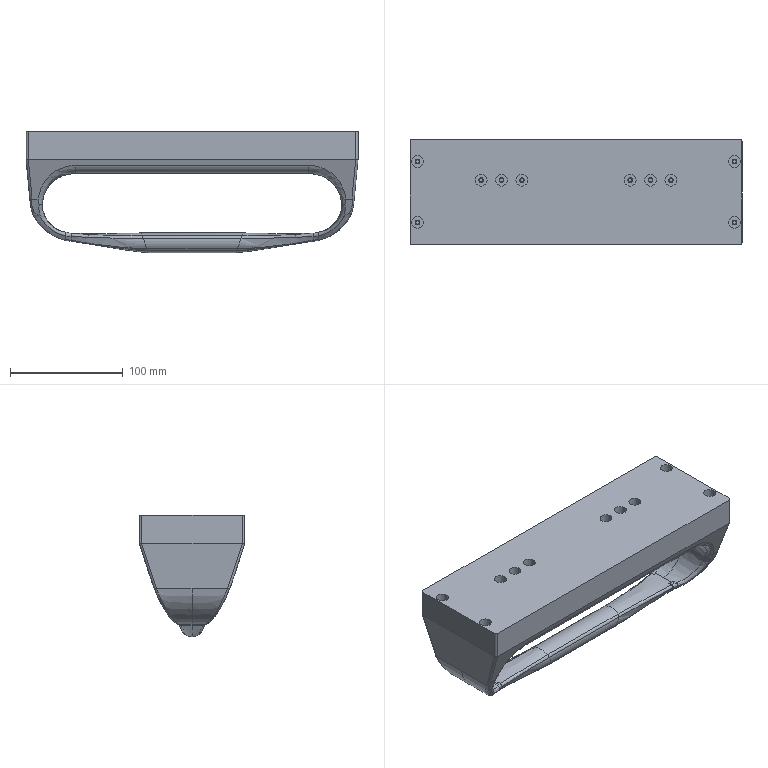NC program | NX | posted with a generic post | part box 294.078 x 93.5 x 107.5 mm
Lines 374 to 1245 of 3753:
(ZLEVEL_PROFILE_COPY_1_COPY_1_COPY_1_1 , TOOL : D6)
N716 T05 M6
N718 G54
N720 G17 G0 G90 X132.194 Y-28.666 B0. C0. S7500 M3
N722 G43 Z28.5 H5
N724 Z-0.05
N726 G94 G1 Z-1.55 F800.
N728 X133.111 Y-28.097
N730 G3 X133.394 Y-27.568 R0.6
N732 G2 X133.414 Y-26.507 R10.372 F3000.
N734 X139.062 Y-20.125 R7.005
N736 G3 X141.389 Y-17.198 R3.024
N738 G1 Y17.198
N740 G3 X138.883 Y20.166 R3.036
N742 G1 X138.816 Y20.183
N744 G2 X133.394 Y27.224 R7.011
N746 G1 Z-1.6
N748 G3 X138.819 Y20.182 R7.011
N750 G1 X138.882 Y20.166
N752 G2 X141.384 Y17.199 R3.035
N754 G1 Y-17.199
N756 G2 X139.062 Y-20.125 R3.024
N758 G3 X133.414 Y-26.507 R7.005
N760 X133.394 Y-27.568 R10.367
N762 G1 Z-1.649
N764 G2 X133.415 Y-26.492 R10.363
N766 X138.873 Y-20.168 R6.993
N768 G1 X139.062 Y-20.125
N770 G3 X141.38 Y-17.2 R3.024
N772 G1 Y17.2
N774 G3 X138.882 Y20.166 R3.034
N776 G1 X138.821 Y20.182
N778 G2 X133.394 Y27.224 R7.011
N780 G1 Z-1.699
N782 G3 X138.824 Y20.181 R7.011
N784 G1 X138.882 Y20.166
N786 G2 X141.375 Y17.201 R3.033
N788 G1 Y-17.201
N790 G2 X139.061 Y-20.125 R3.025
N792 G1 X138.873 Y-20.168
N794 G3 X133.415 Y-26.493 R6.994
N796 X133.394 Y-27.568 R10.358
N798 G1 Z-1.749
N800 G2 X133.415 Y-26.496 R10.384
N802 X138.873 Y-20.168 R6.995
N804 G1 X139.061 Y-20.125
N806 G3 X141.37 Y-17.202 R3.025
N808 G1 Y17.202
N810 G3 X138.881 Y20.166 R3.033
N812 G1 X138.826 Y20.18
N814 G2 X133.394 Y27.224 R7.011
N816 G1 Z-1.799
N818 G3 X138.829 Y20.179 R7.011
N820 G1 X138.881 Y20.166
N822 G2 X141.365 Y17.203 R3.032
N824 G1 Y-17.203
N826 G2 X139.061 Y-20.125 R3.025
N828 G1 X138.873 Y-20.168
N830 G3 X133.415 Y-26.496 R6.995
N832 X133.394 Y-27.568 R10.38
N834 G1 Z-1.848
N836 G2 X133.415 Y-26.496 R10.375
N838 X138.873 Y-20.168 R6.995
N840 G1 X139.061 Y-20.125
N842 G3 X141.361 Y-17.204 R3.025
N844 G1 Y17.204
N846 G3 X138.88 Y20.166 R3.031
N848 G1 X138.831 Y20.179
N850 G2 X133.394 Y27.224 R7.011
N852 G1 Z-1.898
N854 G3 X138.834 Y20.178 R7.011
N856 G1 X138.88 Y20.166
N858 G2 X141.356 Y17.205 R3.03
N860 G1 Y-17.205
N862 G2 X139.06 Y-20.125 R3.025
N864 G1 X138.873 Y-20.168
N866 G3 X133.415 Y-26.496 R6.995
N868 X133.394 Y-27.568 R10.37
N870 G1 Z-1.948
N872 G2 X133.415 Y-26.496 R10.366
N874 X138.873 Y-20.168 R6.995
N876 G1 X139.059 Y-20.125
N878 G3 X141.351 Y-17.206 R3.025
N880 G1 Y17.206
N882 G3 X138.88 Y20.166 R3.03
N884 G1 X138.836 Y20.177
N886 G2 X133.394 Y27.224 R7.011
N888 G1 Z-1.998
N890 G3 X138.839 Y20.176 R7.011
N892 G1 X138.879 Y20.166
N894 G2 X141.346 Y17.207 R3.029
N896 G1 Y-17.207
N898 G2 X139.058 Y-20.125 R3.024
N900 G1 X138.873 Y-20.168
N902 G3 X133.415 Y-26.496 R6.995
N904 X133.394 Y-27.568 R10.361
N906 G1 Z-2.047
N908 G2 X133.415 Y-26.496 R10.356
N910 X138.873 Y-20.168 R6.996
N912 G1 X139.057 Y-20.125
N914 G3 X141.341 Y-17.208 R3.024
N916 G1 Y17.208
N918 G3 X138.879 Y20.166 R3.029
N920 G1 X138.841 Y20.176
N922 G2 X133.394 Y27.224 R7.012
N924 G1 Z-2.097
N926 G3 X138.844 Y20.175 R7.012
N928 G1 X138.878 Y20.166
N930 G2 X141.337 Y17.209 R3.028
N932 G1 Y-17.209
N934 G2 X138.873 Y-20.168 R3.03
N936 G3 X133.415 Y-26.496 R6.996
N938 X133.394 Y-27.568 R10.352
N940 G1 Z-2.147
N942 G2 X133.416 Y-26.488 R10.347
N944 X138.933 Y-20.156 R6.991
N946 G3 X141.332 Y-17.21 R3.03
N948 G1 Y17.21
N950 G3 X138.878 Y20.166 R3.028
N952 G1 X138.846 Y20.174
N954 G2 X133.394 Y27.224 R7.013
N956 G1 Z-2.197
N958 G3 X138.849 Y20.173 R7.013
N960 G1 X138.877 Y20.166
N962 G2 X141.327 Y17.211 R3.027
N964 G1 Y-17.211
N966 G2 X138.93 Y-20.156 R3.029
N968 G3 X133.416 Y-26.488 R6.992
N970 X133.394 Y-27.568 R10.342
N972 G1 Z-2.247
N974 G2 X133.416 Y-26.489 R10.338
N976 X138.927 Y-20.157 R6.992
N978 G3 X141.322 Y-17.212 R3.029
N980 G1 Y17.212
N982 G3 X138.877 Y20.166 R3.026
N984 G1 X138.851 Y20.173
N986 G2 X133.394 Y27.224 R7.014
N988 G1 Z-2.296
N990 G3 X138.877 Y20.166 R7.015
N992 G2 X141.318 Y17.213 R3.026
N994 G1 Y-17.213
N996 G2 X138.924 Y-20.157 R3.029
N998 G3 X133.416 Y-26.489 R6.993
N1000 X133.394 Y-27.568 R10.333
N1002 G1 Z-2.346
N1004 G2 X133.416 Y-26.489 R10.328
N1006 X138.921 Y-20.158 R6.993
N1008 G3 X141.313 Y-17.214 R3.028
N1010 G1 Y17.214
N1012 G3 X138.876 Y20.166 R3.025
N1014 G1 X138.856 Y20.171
N1016 G2 X133.394 Y27.224 R7.015
N1018 G1 Z-2.396
N1020 G3 X138.876 Y20.166 R7.016
N1022 G2 X141.308 Y17.215 R3.025
N1024 G1 Y-17.215
N1026 G2 X138.918 Y-20.158 R3.027
N1028 G3 X133.415 Y-26.49 R6.993
N1030 X133.394 Y-27.568 R10.324
N1032 G1 Z-2.446
N1034 G2 X133.415 Y-26.49 R10.319
N1036 X138.915 Y-20.159 R6.994
N1038 G3 X141.303 Y-17.216 R3.027
N1040 G1 Y17.216
N1042 G3 X138.861 Y20.169 R3.025
N1044 G2 X133.394 Y27.224 R7.016
N1046 G1 Z-2.495
N1048 G3 X138.875 Y20.166 R7.016
N1050 G2 X141.299 Y17.217 R3.024
N1052 G1 Y-17.217
N1054 G2 X138.912 Y-20.159 R3.027
N1056 G3 X133.415 Y-26.491 R6.994
N1058 X133.394 Y-27.568 R10.314
N1060 G1 Z-2.545
N1062 G2 X133.415 Y-26.491 R10.31
N1064 X138.909 Y-20.16 R6.995
N1066 G3 X141.294 Y-17.218 R3.027
N1068 G1 Y17.218
N1070 G3 X138.866 Y20.168 R3.023
N1072 G2 X133.394 Y27.224 R7.017
N1074 G1 Z-2.595
N1076 G3 X138.874 Y20.166 R7.018
N1078 G2 X141.289 Y17.219 R3.022
N1080 G1 Y-17.219
N1082 G2 X138.906 Y-20.16 R3.026
N1084 G3 X133.415 Y-26.492 R6.995
N1086 X133.394 Y-27.568 R10.305
N1088 G1 Z-2.645
N1090 G2 X133.415 Y-26.492 R10.3
N1092 X138.903 Y-20.161 R6.995
N1094 G3 X141.284 Y-17.22 R3.025
N1096 G1 Y17.22
N1098 G3 X138.871 Y20.166 R3.022
N1100 G2 X133.394 Y27.224 R7.018
N1102 G1 Z-2.695
N1104 G3 X138.887 Y20.163 R7.018
N1106 G2 X141.28 Y17.221 R3.021
N1108 G1 Y-17.221
N1110 G2 X138.9 Y-20.161 R3.025
N1112 G3 X133.415 Y-26.493 R6.996
N1114 X133.394 Y-27.568 R10.308
N1116 G1 Z-2.744
N1118 G2 X133.49 Y-25.845 R9.094
N1120 X139.044 Y-20.125 R7.035
N1122 G3 X141.275 Y-17.223 R3.02
N1124 G1 Y17.222
N1126 G3 X138.887 Y20.163 R3.021
N1128 G2 X133.394 Y27.224 R7.017
N1130 G1 Z-2.794
N1132 G3 X138.887 Y20.163 R7.017
N1134 G2 X141.27 Y17.223 R3.02
N1136 G1 Y-17.222
N1138 G2 X141.249 Y-17.572 R2.907
N1140 X139.043 Y-20.125 R3.023
N1142 G3 X133.49 Y-25.845 R7.037
N1144 X133.394 Y-27.568 R9.093
N1146 G1 Z-2.844
N1148 G2 X133.642 Y-25.155 R8.099
N1150 X139.042 Y-20.125 R7.044
N1152 G3 X141.244 Y-17.572 R3.022
N1154 X141.265 Y-17.223 R2.914
N1156 G1 Y17.224
N1158 G3 X138.887 Y20.163 R3.02
N1160 G2 X133.394 Y27.224 R7.017
N1162 G1 Z-2.894
N1164 G3 X138.886 Y20.163 R7.017
N1166 G2 X141.26 Y17.226 R3.019
N1168 G1 Y-17.223
N1170 G2 X141.239 Y-17.575 R2.919
N1172 X139.041 Y-20.125 R3.022
N1174 G3 X133.642 Y-25.155 R7.046
N1176 X133.394 Y-27.568 R8.097
N1178 G1 Z-2.943
N1180 G2 X133.642 Y-25.155 R8.095
N1182 X139.04 Y-20.125 R7.049
N1184 G3 X141.235 Y-17.575 R3.022
N1186 X141.256 Y-17.224 R2.92
N1188 G1 Y17.227
N1190 G3 X138.886 Y20.162 R3.019
N1192 G2 X133.394 Y27.224 R7.019
N1194 G1 Z-2.993
N1196 G3 X138.886 Y20.162 R7.019
N1198 G2 X141.251 Y17.228 R3.019
N1200 G1 Y-17.116
N1202 G2 X141.243 Y-17.388 R4.875
N1204 X138.885 Y-20.163 R3.014
N1206 G3 X133.415 Y-26.5 R7.001
N1208 X133.394 Y-27.568 R10.289
N1210 G1 Z-3.043
N1212 G2 X133.414 Y-26.503 R10.286
N1214 X138.884 Y-20.162 R7.004
N1216 G3 X141.238 Y-17.392 R3.011
N1218 X141.246 Y-17.116 R4.903
N1220 G1 Y17.229
N1222 G3 X138.873 Y20.165 R3.019
N1224 G2 X133.394 Y27.224 R7.019
N1226 G1 Z-3.093
N1228 G3 X138.873 Y20.165 R7.019
N1230 G2 X141.241 Y17.23 R3.019
N1232 G1 Y-17.118
N1234 G2 X141.234 Y-17.392 R4.895
N1236 X138.881 Y-20.163 R3.011
N1238 G3 X133.414 Y-26.504 R7.004
N1240 X133.394 Y-27.568 R10.283
N1242 G1 Z-3.142
N1244 G2 X133.414 Y-26.504 R10.28
N1246 X138.878 Y-20.163 R7.005
N1248 G3 X141.229 Y-17.393 R3.011
N1250 X141.237 Y-17.119 R4.913
N1252 G1 Y17.231
N1254 G3 X138.873 Y20.165 R3.019
N1256 G2 X133.394 Y27.224 R7.019
N1258 G1 Z-3.192
N1260 G3 X138.873 Y20.165 R7.019
N1262 G2 X141.232 Y17.232 R3.018
N1264 G1 Y-17.119
N1266 G2 X141.224 Y-17.393 R4.931
N1268 X138.875 Y-20.164 R3.011
N1270 G3 X133.414 Y-26.505 R7.005
N1272 X133.394 Y-27.568 R10.277
N1274 G1 Z-3.242
N1276 G2 X133.414 Y-26.505 R10.274
N1278 X138.871 Y-20.165 R7.005
N1280 G3 X141.219 Y-17.394 R3.01
N1282 X141.227 Y-17.12 R4.949
N1284 G1 Y17.233
N1286 G3 X138.886 Y20.162 R3.018
N1288 G2 X133.394 Y27.224 R7.02
N1290 G1 Z-3.292
N1292 G3 X138.886 Y20.162 R7.02
N1294 G2 X141.222 Y17.234 R3.017
N1296 G1 Y-17.12
N1298 G2 X141.215 Y-17.394 R4.968
N1300 X138.868 Y-20.165 R3.01
N1302 G3 X133.414 Y-26.505 R7.005
N1304 X133.394 Y-27.568 R10.271
N1306 G1 Z-3.342
N1308 G2 X133.414 Y-26.506 R10.268
N1310 X138.865 Y-20.166 R7.006
N1312 G3 X141.21 Y-17.395 R3.01
N1314 X141.218 Y-17.121 R4.986
N1316 G1 Y17.235
N1318 G3 X138.886 Y20.161 R3.017
N1320 G2 X133.394 Y27.224 R7.021
N1322 G1 Z-3.391
N1324 G3 X138.886 Y20.161 R7.021
N1326 G2 X141.213 Y17.236 R3.017
N1328 G1 Y-17.121
N1330 G2 X141.205 Y-17.396 R5.004
N1332 X138.862 Y-20.167 R3.01
N1334 G3 X133.414 Y-26.506 R7.006
N1336 X133.394 Y-27.568 R10.265
N1338 G1 Z-3.441
N1340 G2 X133.414 Y-26.506 R10.261
N1342 X138.858 Y-20.168 R7.006
N1344 G3 X141.208 Y-17.23 R3.015
N1346 G1 Y17.237
N1348 G3 X138.886 Y20.161 R3.017
N1350 G2 X133.394 Y27.224 R7.021
N1352 G1 Z-3.491
N1354 G3 X138.886 Y20.161 R7.022
N1356 G2 X141.203 Y17.238 R3.017
N1358 G1 Y-17.23
N1360 G2 X138.854 Y-20.168 R3.015
N1362 G3 X133.414 Y-26.507 R7.006
N1364 X133.394 Y-27.568 R10.258
N1366 G1 Z-3.541
N1368 G2 X133.414 Y-26.507 R10.255
N1370 X138.851 Y-20.169 R7.007
N1372 G3 X141.198 Y-17.23 R3.015
N1374 G1 Y17.239
N1376 G3 X138.886 Y20.161 R3.016
N1378 G2 X133.394 Y27.224 R7.022
N1380 G1 Z-3.59
N1382 G3 X138.886 Y20.161 R7.023
N1384 G2 X141.194 Y17.24 R3.016
N1386 G1 Y-17.23
N1388 G2 X138.848 Y-20.17 R3.015
N1390 G3 X133.414 Y-26.507 R7.007
N1392 X133.394 Y-27.568 R10.252
N1394 G1 Z-3.64
N1396 G2 X133.414 Y-26.508 R10.249
N1398 X138.844 Y-20.171 R7.007
N1400 G3 X141.189 Y-17.23 R3.015
N1402 G1 Y17.241
N1404 G3 X138.886 Y20.161 R3.016
N1406 G2 X133.394 Y27.224 R7.023
N1408 G1 Z-3.69
N1410 G3 X138.886 Y20.161 R7.023
N1412 G2 X141.184 Y17.242 R3.016
N1414 G1 Y-17.23
N1416 G2 X138.841 Y-20.171 R3.015
N1418 G3 X133.414 Y-26.508 R7.007
N1420 X133.394 Y-27.568 R10.246
N1422 G1 Z-3.74
N1424 G2 X133.414 Y-26.508 R10.243
N1426 X138.838 Y-20.172 R7.007
N1428 G3 X141.179 Y-17.23 R3.015
N1430 G1 Y17.243
N1432 G3 X138.886 Y20.161 R3.016
N1434 G2 X133.394 Y27.224 R7.023
N1436 G1 Z-3.79
N1438 G3 X138.886 Y20.16 R7.023
N1440 G2 X141.175 Y17.244 R3.016
N1442 G1 Y-17.23
N1444 G2 X139.558 Y-19.905 R3.014
N1446 X138.944 Y-20.145 R2.775
N1448 G1 X138.559 Y-20.245
N1450 G3 X133.415 Y-26.492 R6.995
N1452 X133.394 Y-27.568 R10.24
N1454 G1 Z-3.839
N1456 G2 X133.414 Y-26.516 R10.642
N1458 X138.559 Y-20.245 R6.993
N1460 G1 X138.942 Y-20.146
N1462 G3 X139.558 Y-19.904 R2.767
N1464 X141.17 Y-17.23 R3.014
N1466 G1 Y17.245
N1468 G3 X138.886 Y20.16 R3.016
N1470 G2 X133.394 Y27.224 R7.024
N1472 G1 Z-3.889
N1474 G3 X138.886 Y20.16 R7.024
N1476 G2 X141.165 Y17.246 R3.016
N1478 G1 Y-17.23
N1480 G2 X139.558 Y-19.902 R3.015
N1482 X138.94 Y-20.146 R2.76
N1484 G1 X138.559 Y-20.245
N1486 G3 X133.414 Y-26.516 R6.993
N1488 X133.394 Y-27.568 R10.64
N1490 G1 Z-3.939
N1492 G2 X133.414 Y-26.516 R10.638
N1494 X138.559 Y-20.245 R6.993
N1496 G1 X138.913 Y-20.153
N1498 G3 X139.782 Y-19.77 R2.994
N1500 X141.16 Y-17.23 R3.017
N1502 G1 Y17.247
N1504 G3 X138.886 Y20.16 R3.017
N1506 G2 X133.394 Y27.224 R7.024
N1508 G1 Z-3.989
N1510 G3 X138.886 Y20.16 R7.026
N1512 G2 X141.156 Y17.248 R3.017
N1514 G1 Y-17.23
N1516 G2 X139.81 Y-19.75 R3.017
N1518 X138.91 Y-20.154 R2.993
N1520 G1 X138.559 Y-20.245
N1522 G3 X133.414 Y-26.516 R6.993
N1524 X133.394 Y-27.568 R10.637
N1526 G1 Z-4.038
N1528 G2 X133.413 Y-26.533 R10.635
N1530 X138.817 Y-20.177 R7.006
N1532 G3 X141.151 Y-17.23 R3.016
N1534 G1 Y17.249
N1536 G3 X138.887 Y20.159 R3.016
N1538 G2 X133.394 Y27.224 R7.035
N1540 G1 Z-4.088
N1542 G3 X133.578 Y25.415 R7.245
N1544 X138.811 Y20.178 R6.992
N1546 G2 X141.146 Y17.25 R3.016
N1548 G1 Y-17.23
N1550 G2 X138.814 Y-20.178 R3.016
N1552 G3 X133.413 Y-26.533 R7.006
N1554 X133.394 Y-27.568 R10.633
N1556 G1 Z-4.138
N1558 G2 X133.413 Y-26.533 R10.632
N1560 X138.81 Y-20.178 R7.006
N1562 G3 X141.141 Y-17.23 R3.016
N1564 G1 Y17.251
N1566 G3 X138.887 Y20.159 R3.017
N1568 G2 X133.869 Y24.467 R7.049
N1570 X133.394 Y27.224 R7.164
N1572 G1 Z-4.188
N1574 G3 X133.869 Y24.467 R7.164
N1576 X138.886 Y20.159 R7.052
N1578 G2 X141.136 Y17.252 R3.017
N1580 G1 Y-17.23
N1582 G2 X138.873 Y-20.163 R3.016
N1584 G3 X133.413 Y-26.532 R7.007
N1586 X133.394 Y-27.568 R10.631
N1588 G1 Z-4.237
N1590 G2 X133.413 Y-26.532 R10.63
N1592 X138.873 Y-20.163 R7.007
N1594 G3 X141.132 Y-17.23 R3.017
N1596 G1 Y17.253
N1598 G3 X138.886 Y20.159 R3.017
N1600 G2 X133.91 Y24.363 R7.056
N1602 X133.394 Y27.224 R7.142
N1604 G1 Z-4.287
N1606 G3 X134.181 Y23.778 R7.096
N1608 X138.885 Y20.159 R7.066
N1610 G2 X141.127 Y17.255 R3.017
N1612 G1 Y-17.23
N1614 G2 X138.873 Y-20.163 R3.017
N1616 G3 X133.413 Y-26.533 R7.007
N1618 X133.394 Y-27.568 R10.629
N1620 G1 Z-4.337
N1622 G2 X133.413 Y-26.533 R10.628
N1624 X138.873 Y-20.163 R7.007
N1626 G3 X141.122 Y-17.23 R3.017
N1628 G1 Y17.256
N1630 G3 X138.885 Y20.159 R3.016
N1632 G1 X138.584 Y20.24
N1634 G2 X133.394 Y27.224 R7.012
N1636 G1 Z-4.387
N1638 G3 X138.581 Y20.241 R7.012
N1640 G1 X138.884 Y20.159
N1642 G2 X141.117 Y17.257 R3.017
N1644 G1 Y-17.23
N1646 G2 X138.873 Y-20.163 R3.017
N1648 G3 X133.413 Y-26.533 R7.008
N1650 X133.394 Y-27.568 R10.627
N1652 G1 Z-4.437
N1654 G2 X133.413 Y-26.534 R10.625
N1656 X138.873 Y-20.163 R7.008
N1658 G3 X141.113 Y-17.23 R3.017
N1660 G1 Y17.258
N1662 G3 X138.884 Y20.159 R3.017
N1664 G1 X138.579 Y20.242
N1666 G2 X133.394 Y27.224 R7.012
N1668 G1 Z-4.486
N1670 G3 X138.576 Y20.242 R7.012
N1672 G1 X138.883 Y20.159
N1674 G2 X141.108 Y17.259 R3.017
N1676 G1 Y-17.23
N1678 G2 X138.873 Y-20.162 R3.017
N1680 G3 X133.413 Y-26.535 R7.008
N1682 X133.394 Y-27.568 R10.624
N1684 G1 Z-4.536
N1686 G2 X133.412 Y-26.535 R10.622
N1688 X138.873 Y-20.162 R7.009
N1690 G3 X141.103 Y-17.23 R3.017
N1692 G1 Y17.26
N1694 G3 X138.883 Y20.159 R3.017
N1696 G1 X138.573 Y20.243
N1698 G2 X133.394 Y27.224 R7.012
N1700 G1 Z-4.586
N1702 G3 X138.57 Y20.244 R7.012
N1704 G1 X138.882 Y20.159
N1706 G2 X141.098 Y17.261 R3.017
N1708 G1 Y-17.23
N1710 G2 X138.873 Y-20.162 R3.017
N1712 G3 X133.441 Y-26.19 R7.02
N1714 X133.394 Y-27.568 R10.621
N1716 G1 Z-4.636
N1718 X133.397 Y-26.818
N1720 X133.4 Y-26.707
N1722 G2 X138.873 Y-20.162 R7.017
N1724 G3 X141.094 Y-17.23 R3.017
N1726 G1 Y17.262
N1728 G3 X138.882 Y20.159 R3.018
N1730 G1 X138.567 Y20.245
N1732 G2 X133.394 Y27.224 R7.012
N1734 G1 Z-4.685
N1736 G3 X138.565 Y20.245 R7.013
N1738 G1 X138.881 Y20.159
N1740 G2 X141.089 Y17.263 R3.018
N1742 G1 Y-17.23
N1744 G2 X138.873 Y-20.162 R3.018
N1746 G3 X133.4 Y-26.707 R7.018
N1748 G1 X133.397 Y-26.818
N1750 X133.394 Y-27.568
N1752 Z-4.735
N1754 X133.397 Y-26.818
N1756 X133.4 Y-26.707
N1758 G2 X138.873 Y-20.162 R7.022
N1760 G3 X141.084 Y-17.23 R3.018
N1762 G1 Y17.264
N1764 G3 X138.702 Y20.208 R3.03
N1766 G2 X133.394 Y27.224 R7.013
N1768 G1 Z-4.785
N1770 G3 X138.702 Y20.208 R7.013
N1772 G2 X141.079 Y17.265 R3.029
N1774 G1 Y-17.23
N1776 G2 X138.873 Y-20.162 R3.018
N1778 G3 X133.4 Y-26.707 R7.026
N1780 G1 X133.397 Y-26.818
N1782 X133.394 Y-27.568
N1784 Z-4.835
N1786 G2 X133.441 Y-26.19 R11.372
N1788 X138.873 Y-20.161 R7.032
N1790 G3 X141.074 Y-17.23 R3.019
N1792 G1 Y17.266
N1794 G3 X138.702 Y20.208 R3.029
N1796 G2 X133.394 Y27.224 R7.013
N1798 G1 Z-4.885
N1800 G3 X138.702 Y20.208 R7.013
N1802 G2 X141.07 Y17.268 R3.028
N1804 G1 Y-17.23
N1806 G2 X138.873 Y-20.161 R3.019
N1808 G3 X133.441 Y-26.19 R7.036
N1810 X133.394 Y-27.568 R11.371
N1812 G1 Z-4.934
N1814 X133.397 Y-26.818
N1816 X133.4 Y-26.707
N1818 G2 X138.558 Y-20.245 R7.001
N1820 G1 X138.873 Y-20.161
N1822 G3 X139.65 Y-19.815 R3.053
N1824 X141.065 Y-17.23 R3.016
N1826 G1 Y17.269
N1828 G3 X138.702 Y20.208 R3.028
N1830 G2 X133.394 Y27.224 R7.013
N1832 G1 Z-4.984
N1834 G3 X138.702 Y20.208 R7.013
N1836 G2 X141.06 Y17.27 R3.028
N1838 G1 Y-17.23
N1840 G2 X139.647 Y-19.815 R3.016
N1842 X138.873 Y-20.161 R3.067
N1844 G1 X138.558 Y-20.245
N1846 G3 X133.4 Y-26.707 R7.001
N1848 G1 X133.397 Y-26.818
N1850 X133.394 Y-27.568
N1852 Z-5.034
N1854 X133.397 Y-26.818
N1856 X133.4 Y-26.707
N1858 G2 X138.558 Y-20.245 R7.001
N1860 G1 X138.873 Y-20.161
N1862 G3 X139.644 Y-19.815 R3.076
N1864 X141.055 Y-17.23 R3.015
N1866 G1 Y17.271
N1868 G3 X138.702 Y20.208 R3.027
N1870 G2 X133.394 Y27.224 R7.013
N1872 G1 Z-5.084
N1874 G3 X138.702 Y20.208 R7.013
N1876 G2 X141.051 Y17.272 R3.027
N1878 G1 Y-17.23
N1880 G2 X139.641 Y-19.815 R3.015
N1882 X138.873 Y-20.161 R3.052
N1884 G1 X138.558 Y-20.245
N1886 G3 X133.4 Y-26.707 R7.001
N1888 G1 X133.397 Y-26.818
N1890 X133.394 Y-27.568
N1892 Z-5.133
N1894 X133.397 Y-26.818
N1896 X133.4 Y-26.707
N1898 G2 X138.558 Y-20.245 R7.002
N1900 G1 X138.873 Y-20.16
N1902 G3 X139.885 Y-19.642 R3.092
N1904 X141.046 Y-17.23 R3.019
N1906 G1 Y17.273
N1908 G3 X138.787 Y20.184 R3.019
N1910 G2 X133.394 Y27.224 R7.021
N1912 G1 Z-5.183
N1914 G3 X138.787 Y20.184 R7.021
N1916 G2 X141.041 Y17.275 R3.019
N1918 G1 Y-17.23
N1920 G2 X140.257 Y-19.292 R3.009
N1922 X138.728 Y-20.202 R3.051
N1924 G3 X133.4 Y-26.707 R7.002
N1926 G1 X133.397 Y-26.818
N1928 X133.394 Y-27.568
N1930 Z-5.233
N1932 X133.397 Y-26.818
N1934 X133.4 Y-26.707
N1936 G2 X138.558 Y-20.245 R7.002
N1938 G1 X138.805 Y-20.179
N1940 G3 X140.453 Y-19.049 R3.023
N1942 X141.036 Y-17.23 R3.012
N1944 G1 Y17.276
N1946 G3 X138.786 Y20.184 R3.019
N1948 G2 X133.394 Y27.224 R7.021
N1950 G1 Z-5.283
N1952 G3 X138.702 Y20.208 R7.013
N1954 G2 X141.032 Y17.277 R3.026
N1956 G1 Y-17.23
N1958 G2 X140.222 Y-19.323 R3.013
N1960 X138.8 Y-20.18 R3.027
N1962 G1 X138.558 Y-20.245
N1964 G3 X133.4 Y-26.707 R7.002
N1966 G1 X133.397 Y-26.818
N1968 X133.394 Y-27.568
N1970 Z-5.332
N1972 X133.397 Y-26.818
N1974 X133.4 Y-26.707
N1976 G2 X138.558 Y-20.245 R7.002
N1978 G1 X138.797 Y-20.181
N1980 G3 X141.027 Y-17.265 R3.021
N1982 G1 Y17.278
N1984 G3 X138.702 Y20.208 R3.026
N1986 G2 X133.394 Y27.224 R7.013
N1988 G1 Z-5.382
N1990 G3 X138.702 Y20.208 R7.014
N1992 G2 X141.022 Y17.279 R3.026
N1994 G1 Y-17.265
N1996 G2 X138.792 Y-20.182 R3.023
N1998 G1 X138.558 Y-20.245
N2000 G3 X133.4 Y-26.707 R7.002
N2002 G1 X133.397 Y-26.822
N2004 X133.394 Y-27.568
N2006 Z-5.432
N2008 X133.397 Y-26.822
N2010 X133.4 Y-26.707
N2012 G2 X138.558 Y-20.245 R7.002
N2014 G1 X138.792 Y-20.182
N2016 G3 X140.71 Y-18.598 R3.021
N2018 X141.017 Y-17.275 R3.003
N2020 G1 Y17.28
N2022 G3 X138.701 Y20.207 R3.026
N2024 G2 X133.394 Y27.224 R7.014
N2026 G1 Z-5.482
N2028 G3 X138.701 Y20.207 R7.014
N2030 G2 X141.013 Y17.282 R3.026
N2032 G1 Y-17.278
N2034 G2 X140.705 Y-18.6 R2.996
N2036 X138.786 Y-20.183 R3.025
N2038 G1 X138.558 Y-20.245
N2040 G3 X133.4 Y-26.707 R7.002
N2042 G1 X133.397 Y-26.822
N2044 X133.394 Y-27.568
N2046 Z-5.532
N2048 X133.397 Y-26.822
N2050 X133.4 Y-26.707
N2052 G2 X138.558 Y-20.245 R7.002
N2054 G1 X138.782 Y-20.184
N2056 G3 X140.696 Y-18.609 R3.027
N2058 X141.008 Y-17.28 R2.992
N2060 G1 Y17.283
N2062 G3 X138.701 Y20.207 R3.026
N2064 G2 X133.394 Y27.224 R7.014
N2066 G1 Z-5.581
N2068 G3 X138.701 Y20.207 R7.014
N2070 G2 X141.003 Y17.284 R3.026
N2072 G1 Y-17.281
N2074 G2 X140.692 Y-18.609 R2.991
N2076 X138.779 Y-20.185 R3.028
N2078 G1 X138.558 Y-20.245
N2080 G3 X133.4 Y-26.707 R7.002
N2082 G1 X133.397 Y-26.822
N2084 X133.394 Y-27.568
N2086 Z-5.631
N2088 X133.397 Y-26.822
N2090 X133.4 Y-26.707
N2092 G2 X138.558 Y-20.245 R7.002
N2094 G1 X138.777 Y-20.185
N2096 G3 X140.688 Y-18.609 R3.027
N2098 X140.998 Y-17.282 R2.992
N2100 G1 Y17.285
N2102 G3 X138.701 Y20.207 R3.026
N2104 G2 X133.394 Y27.224 R7.014
N2106 G1 Z-5.681
N2108 G3 X138.701 Y20.207 R7.015
N2110 G2 X140.993 Y17.286 R3.026
N2112 G1 Y-17.284
N2114 G2 X140.684 Y-18.609 R2.987
N2116 X138.774 Y-20.186 R3.03
N2118 G1 X138.558 Y-20.245
N2120 G3 X133.4 Y-26.707 R7.002
N2122 G1 X133.397 Y-26.822
N2124 X133.394 Y-27.568
N2126 Z-5.731
N2128 X133.397 Y-26.822
N2130 X133.4 Y-26.707
N2132 G2 X138.558 Y-20.245 R7.002
N2134 G1 X138.772 Y-20.186
N2136 G3 X140.989 Y-17.279 R3.024
N2138 G1 Y-17.23
N2140 Y17.287
N2142 G3 X138.701 Y20.207 R3.025
N2144 G2 X133.394 Y27.224 R7.015
N2146 G1 Z-5.78
N2148 G3 X138.701 Y20.207 R7.015
N2150 G2 X140.984 Y17.289 R3.026
N2152 G1 Y-17.23
N2154 Y-17.282
N2156 G2 X138.769 Y-20.187 R3.026
N2158 G1 X138.558 Y-20.245
N2160 G3 X133.4 Y-26.707 R7.002
N2162 G1 X133.397 Y-26.822
N2164 X133.394 Y-27.568
N2166 Z-5.83
N2168 X133.397 Y-26.822
N2170 X133.4 Y-26.707
N2172 G2 X138.558 Y-20.245 R7.002
N2174 G1 X138.77 Y-20.186
N2176 G3 X140.979 Y-17.276 R3.021
N2178 G1 Y17.29
N2180 G3 X138.701 Y20.207 R3.025
N2182 G2 X133.394 Y27.224 R7.015
N2184 G1 Z-5.88
N2186 G3 X138.701 Y20.207 R7.015
N2188 G2 X140.974 Y17.291 R3.026
N2190 G1 Y-17.277
N2192 G2 X138.768 Y-20.187 R3.021
N2194 G1 X138.558 Y-20.245
N2196 G3 X133.4 Y-26.707 R7.002
N2198 G1 X133.397 Y-26.822
N2200 X133.394 Y-27.568
N2202 Z-5.93
N2204 X133.397 Y-26.822
N2206 X133.4 Y-26.707
N2208 G2 X138.558 Y-20.245 R7.002
N2210 G1 X138.766 Y-20.187
N2212 G3 X140.97 Y-17.278 R3.021
N2214 G1 Y17.292
N2216 G3 X138.701 Y20.207 R3.026
N2218 G2 X133.394 Y27.224 R7.015
N2220 G1 Z-5.979
N2222 G3 X138.701 Y20.207 R7.015
N2224 G2 X140.965 Y17.293 R3.026
N2226 G1 Y-17.28
N2228 G2 X138.763 Y-20.187 R3.021
N2230 G1 X138.558 Y-20.245
N2232 G3 X133.4 Y-26.707 R7.002
N2234 G1 X133.397 Y-26.822
N2236 X133.394 Y-27.568
N2238 Z-6.029
N2240 X133.397 Y-26.822
N2242 X133.4 Y-26.707
N2244 G2 X138.558 Y-20.245 R7.002
N2246 G1 X138.762 Y-20.188
N2248 G3 X140.96 Y-17.281 R3.021
N2250 G1 Y17.294
N2252 G3 X138.701 Y20.207 R3.025
N2254 G2 X133.394 Y27.224 R7.015
N2256 G1 Z-6.079
N2258 G3 X138.701 Y20.206 R7.016
N2260 G2 X140.955 Y17.296 R3.025
N2262 G1 Y-17.282
N2264 G2 X138.759 Y-20.188 R3.021
N2266 G1 X138.558 Y-20.245
N2268 G3 X133.4 Y-26.707 R7.002
N2270 G1 X133.397 Y-26.822
N2272 X133.394 Y-27.568
N2274 Z-6.129
N2276 X133.397 Y-26.822
N2278 X133.4 Y-26.707
N2280 G2 X138.558 Y-20.245 R7.002
N2282 G1 X138.757 Y-20.189
N2284 G3 X140.951 Y-17.283 R3.022
N2286 G1 Y17.297
N2288 G3 X138.701 Y20.206 R3.025
N2290 G2 X133.394 Y27.224 R7.016
N2292 G1 Z-6.179
N2294 G3 X138.701 Y20.206 R7.018
N2296 G2 X140.946 Y17.298 R3.024
N2298 G1 Y-17.29
N2300 G2 X138.761 Y-20.187 R3.013
N2302 G1 X138.558 Y-20.245
N2304 G3 X133.4 Y-26.707 R7.002
N2306 G1 X133.397 Y-26.822
N2308 X133.394 Y-27.568
N2310 Z-6.228
N2312 X133.397 Y-26.822
N2314 X133.4 Y-26.707
N2316 G2 X138.558 Y-20.245 R7.002
N2318 G1 X138.759 Y-20.188
N2320 G3 X140.941 Y-17.291 R3.014
N2322 G1 Y17.299
N2324 G3 X138.668 Y20.215 R3.026
N2326 G2 X133.394 Y27.224 R7.026
N2328 G1 Z-6.278
N2330 G3 X138.665 Y20.216 R7.027
N2332 G2 X140.936 Y17.3 R3.026
N2334 G1 Y-17.292
N2336 G2 X138.757 Y-20.188 R3.014
N2338 G1 X138.558 Y-20.245
N2340 G3 X133.4 Y-26.707 R7.002
N2342 G1 X133.397 Y-26.822
N2344 X133.394 Y-27.568
N2346 Z-6.328
N2348 X133.397 Y-26.822
N2350 X133.4 Y-26.707
N2352 G2 X138.557 Y-20.245 R7.002
N2354 G1 X138.755 Y-20.188
N2356 G3 X140.931 Y-17.293 R3.014
N2358 G1 Y17.301
N2360 G3 X138.662 Y20.216 R3.026
N2362 G2 X133.394 Y27.224 R7.028
N2364 G1 Z-6.378
N2366 G3 X138.786 Y20.181 R7.03
N2368 G2 X140.927 Y17.23 R3.027
N2370 G1 Y-17.294
N2372 G2 X138.753 Y-20.189 R3.014
N2374 G1 X138.557 Y-20.245
N2376 G3 X133.4 Y-26.707 R7.002
N2378 G1 X133.397 Y-26.822
N2380 X133.394 Y-27.568
N2382 Z-6.427
N2384 X133.397 Y-26.822
N2386 X133.4 Y-26.707
N2388 G2 X138.557 Y-20.245 R7.002
N2390 G1 X138.751 Y-20.189
N2392 G3 X140.922 Y-17.296 R3.014
N2394 G1 Y17.23
N2396 G3 X138.785 Y20.181 R3.026
N2398 G2 X133.394 Y27.224 R7.037
N2400 G1 Z-6.477
N2402 G3 X133.507 Y25.756 R7.121
N2404 X138.651 Y20.219 R7.02
N2406 G2 X140.917 Y17.23 R3.026
N2408 G1 Y-17.297
N2410 G2 X138.75 Y-20.189 R3.014
N2412 G1 X138.557 Y-20.245
N2414 G3 X133.4 Y-26.707 R7.002
N2416 G1 X133.397 Y-26.822
N2418 X133.394 Y-27.568
N2420 Z-6.527
N2422 X133.397 Y-26.822
N2424 X133.4 Y-26.707
N2426 G2 X138.557 Y-20.245 R7.002
N2428 G1 X138.748 Y-20.19
N2430 G3 X140.912 Y-17.298 R3.014
N2432 G1 Y17.23
N2434 G3 X138.785 Y20.18 R3.026
N2436 G2 X134.623 Y23.039 R7.105
N2438 X133.394 Y27.224 R7.053
N2440 G1 Z-6.577
N2442 G3 X135.06 Y22.468 R7.037
N2444 X138.785 Y20.18 R7.147
N2446 G2 X140.908 Y17.23 R3.025
N2448 G1 Y-17.296
N2450 G2 X138.743 Y-20.191 R3.018
N2452 G1 X138.557 Y-20.245